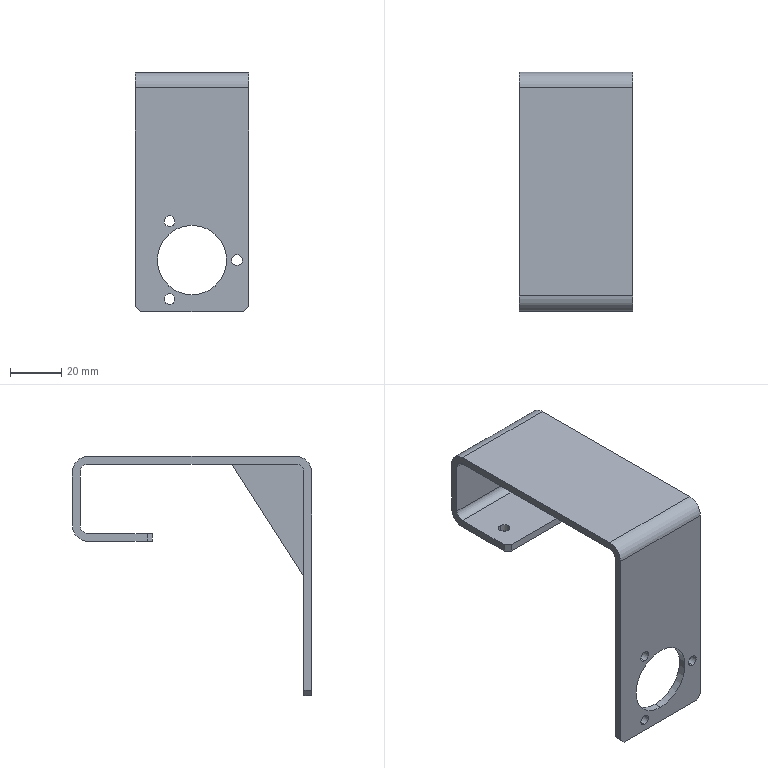Part | STEP file | rotary joint support 2_SUS304 | 1 solid | 38 faces | box 44 x 93 x 93 mm | volume 30917 mm3 | cylinder 19 | plane 19 | commonest cylinder face diameters 4.2 x6 4.5 x4 6 x4 12 x3 27 x2